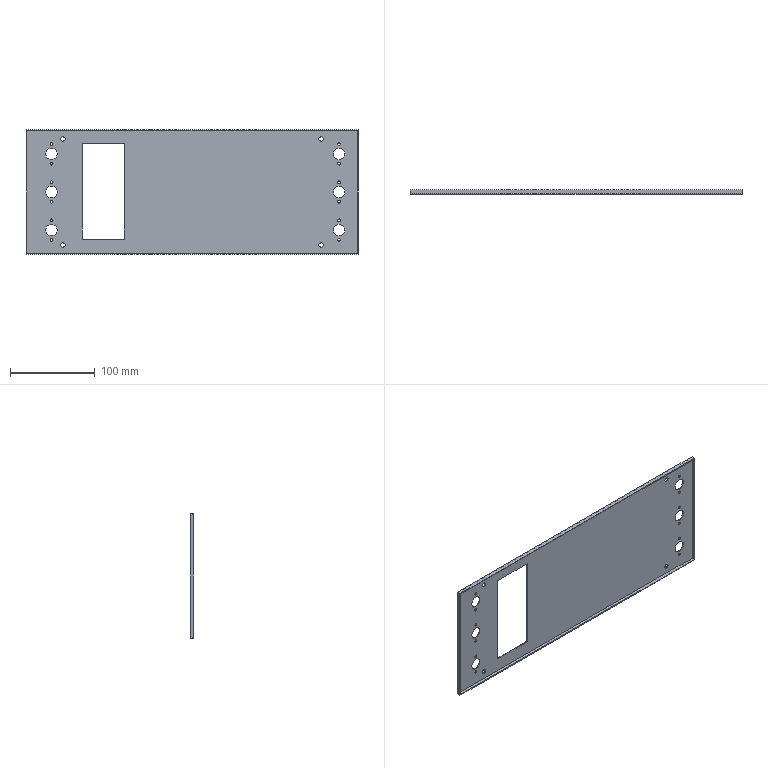Part | SolidWorks | features MoveFace 8, ICE 5, Cut 1, Extrusion 1 | 1 solid | 59 faces | box 392.4 x 4.5 x 147.15 mm | volume 54814 mm3 | cylinder 44 | plane 15 | commonest cylinder face diameters 3.2 x24 13.5 x12 5.2 x8